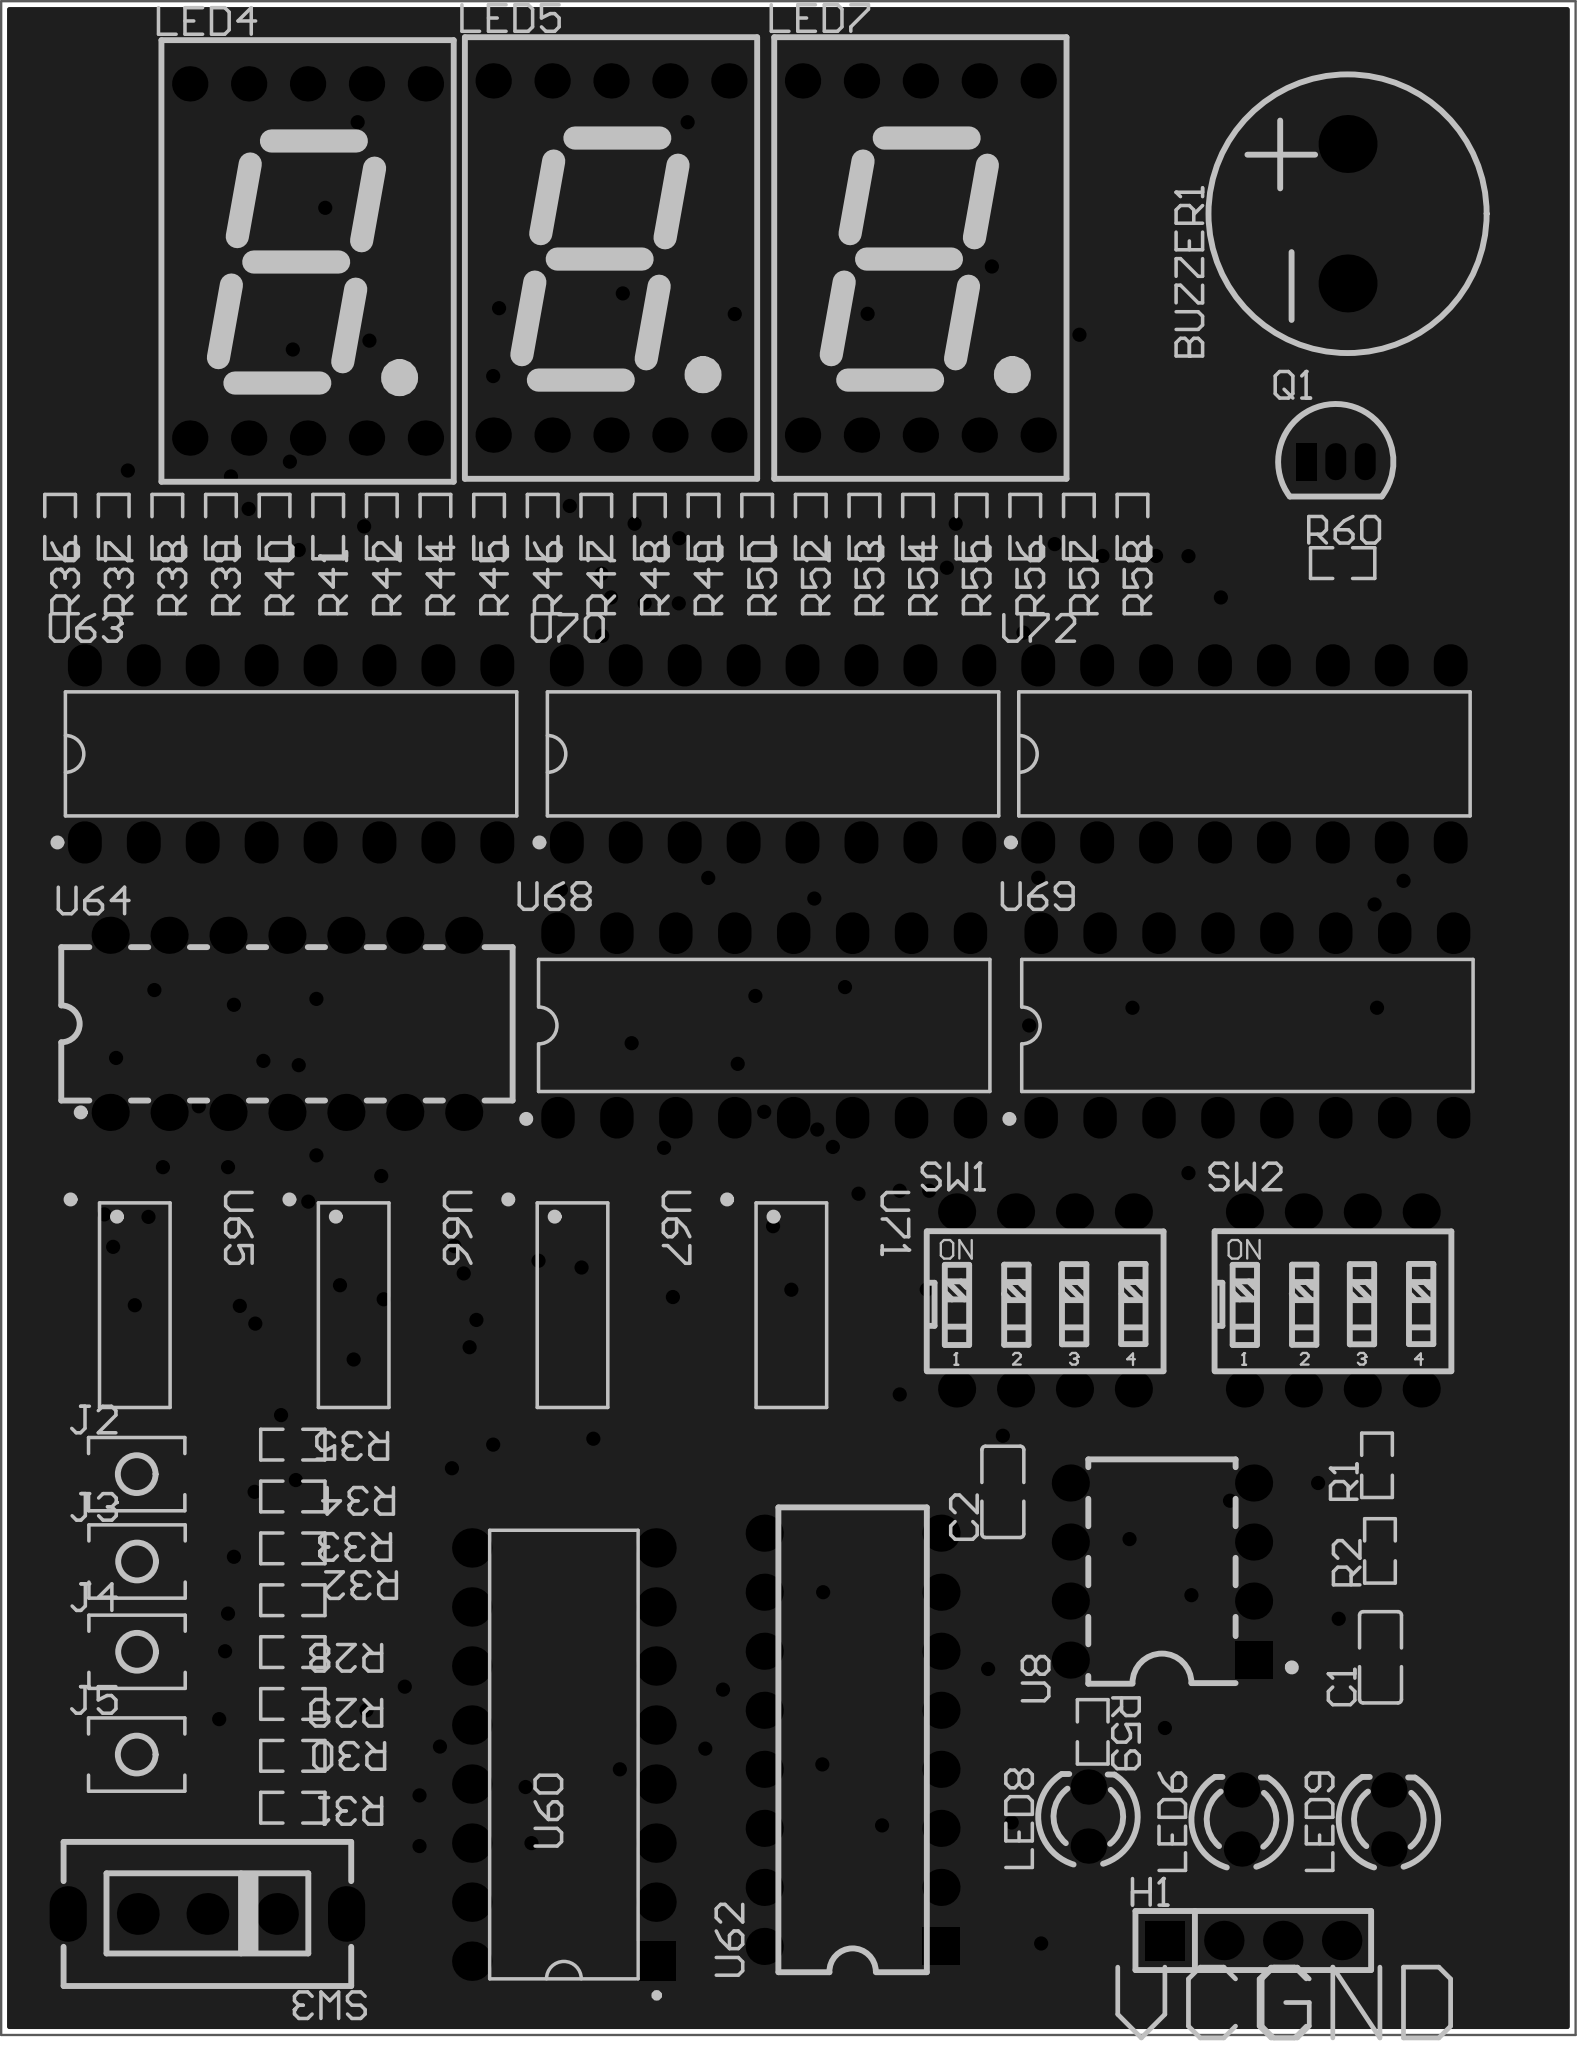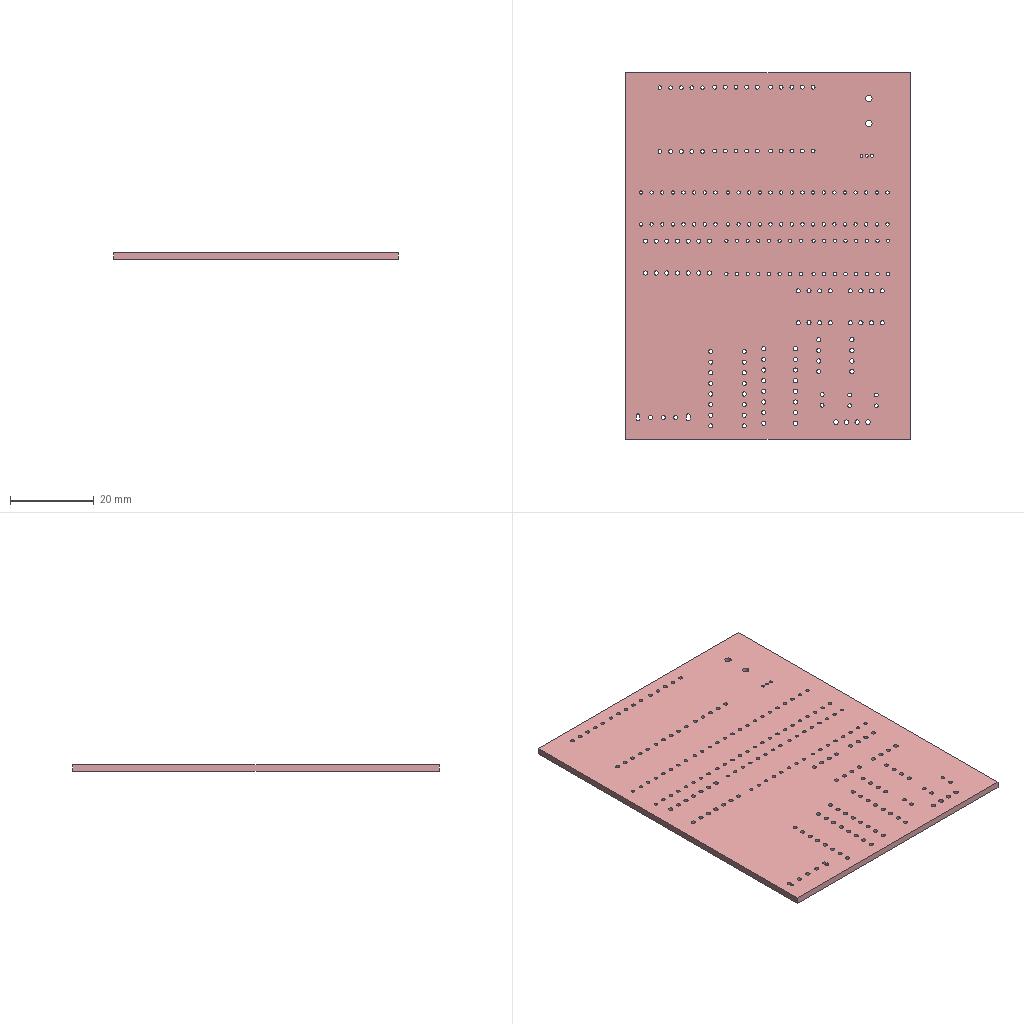Circuit board layout | Altium Designer | box 67.9 x 87.5 x 1.6 mm
Layer stack:
# Altium Designer layer stack of  (unit mm; dielectric type: 0 none, 1 core, 2 prepreg, 3 surface material)
index,name,kind,layer,copper_thickness_mm,dielectric_type,dielectric_thickness_mm,dielectric_material,dielectric_constant
0,Top Paste Mask Layer,other,,,,,,
1,Top Silkscreen Layer,other,,,,,,
2,Top Solder Mask Layer,dielectric,,,3,0.01,,3.3
3,Top Layer,copper,Top Layer,0.035,,,,
4,Dielectric1,dielectric,,,3,1.51,FR4,4.5
5,Bottom Layer,copper,Bottom Layer,0.035,,,,
6,Bottom Solder Mask Layer,dielectric,,,3,0.01,,3.3
7,Bottom Silkscreen Layer,other,,,,,,
8,Bottom Paste Mask Layer,other,,,,,,
# drill layer pairs: low layer,high layer
drill_pair,Top Layer,Bottom Layer
Part placement:
Designator,Comment,Layer,Footprint,Center-X(mm),Center-Y(mm),Rotation
BUZZER1,buzzer,TopLayer,BUZ-TH_BD12.0-P6.00-D0.9-RD,137.668,157.099,90
C1,100uF,TopLayer,C0805,139.089,94.989,90
C2,10nF,TopLayer,C0805,122.809,102.108,90
J2,Tact switch 3*4*H,TopLayer,SW-SMD_L4.0-W2.9-LS5.0,85.471,102.87,0
J3,Tact switch 3*4*H,TopLayer,SW-SMD_L4.0-W2.9-LS5.0,85.486,99.111,0
J4,Tact switch 3*4*H,TopLayer,SW-SMD_L4.0-W2.9-LS5.0,85.486,95.227,0
J5,Tact switch 3*4*H,TopLayer,SW-SMD_L4.0-W2.9-LS5.0,85.471,90.805,0
LED4,,TopLayer,LED-SEG-TH_10P-L12.6-W19.0-P2.54-S15.24-BL,92.837,155.067,0
LED5,,TopLayer,LED-SEG-TH_10P-L12.6-W19.0-P2.54-S15.24-BL,105.918,155.194,0
LED6,,TopLayer,LED_TH-3mm,133.096,88.011,90
LED7,,TopLayer,LED-SEG-TH_10P-L12.6-W19.0-P2.54-S15.24-BL,119.253,155.194,0
LED8,,TopLayer,LED_TH-3mm,126.492,88.138,90
Q1,2N2222A,TopLayer,TO-92-3_L4.9-W3.7-P1.27-L,137.16,146.431,0
R1,10k,TopLayer,R0603,138.938,103.251,90
R2,2.2k,TopLayer,R0603,139.065,99.568,90
R28,10k,TopLayer,R0603,92.202,95.214,180
R29,10k,TopLayer,R0603,92.202,92.982,180
R30,10k,TopLayer,R0603,92.202,90.751,180
R31,10k,TopLayer,R0603,92.202,88.519,180
R32,10k,TopLayer,R0603,92.202,97.445,180
R33,10k,TopLayer,R0603,92.202,99.677,180
R34,10k,TopLayer,R0603,92.202,101.908,180
R35,10k,TopLayer,R0603,92.202,104.14,180
R36,330,TopLayer,R0603,82.169,143.637,90
R37,330,TopLayer,R0603,84.48,143.637,90
R38,330,TopLayer,R0603,86.792,143.637,90
R39,330,TopLayer,R0603,89.103,143.637,90
R40,330,TopLayer,R0603,91.415,143.637,90
R41,330,TopLayer,R0603,93.726,143.637,90
R42,330,TopLayer,R0603,96.037,143.637,90
R44,330,TopLayer,R0603,98.349,143.637,90
R45,330,TopLayer,R0603,100.66,143.637,90
R46,330,TopLayer,R0603,102.972,143.637,90
R47,330,TopLayer,R0603,105.283,143.637,90
R48,330,TopLayer,R0603,107.594,143.637,90
R49,330,TopLayer,R0603,109.906,143.637,90
R50,330,TopLayer,R0603,112.217,143.637,90
R52,330,TopLayer,R0603,114.529,143.637,90
R53,330,TopLayer,R0603,116.84,143.637,90
R54,330,TopLayer,R0603,119.151,143.637,90
R55,330,TopLayer,R0603,121.463,143.637,90
R56,330,TopLayer,R0603,123.774,143.637,90
R57,330,TopLayer,R0603,126.086,143.637,90
R58,330,TopLayer,R0603,128.397,143.637,90
R59,500,TopLayer,R0603,126.681,91.783,270
R60,2k,TopLayer,R0603,137.457,142.066,0
SW1,DIP switch EI-04,TopLayer,SW-TH_DIPSWITCHEI-04,124.625,110.344,0
SW2,DIP switch EI-04,TopLayer,SW-TH_DIPSWITCHEI-04,137.033,110.344,0
U8,NE555PE4,TopLayer,PDIP-8_L9.6-W6.4-P2.54-LS7.9-BL-1,129.667,98.679,90
U60,SN74148N,TopLayer,PDIP-16_L19.3-W6.4-P2.54-LS7.9-BL,103.886,90.805,90
U62,74279N,TopLayer,DIP-16_L19.8-W6.5-P2.54-LS7.6-BL,116.332,91.44,90
U63,SN74LS48N,TopLayer,DIP-16_L19.3-W6.4-P2.54-LS7.6-BL,92.126,133.858,0
U64,SN74LS00N(LX),TopLayer,PDIP-14_L19.3-W6.4-P2.54-LS7.9-BL,91.948,122.244,0
U65,SN74LS04DR,TopLayer,SOIC-14_L8.7-W3.9-P1.27-LS6.0-BL,85.39,110.139,270
U66,SN74LS08DR(LX),TopLayer,SOIC-14_L8.7-W3.9-P1.27-LS6.0-BL,94.824,110.139,270
U67,SN74LS32DR,TopLayer,SOIC-14_L8.7-W3.9-P1.27-LS6.0-BL,104.258,110.139,270
U68,SN74LS192N(LX),TopLayer,PDIP-16_L19.3-W6.4-P2.54-LS7.94-BL,112.522,122.174,0
U69,SN74LS192N(LX),TopLayer,PDIP-16_L19.3-W6.4-P2.54-LS7.94-BL,133.35,122.174,0
U70,SN74LS48N,TopLayer,DIP-16_L19.3-W6.4-P2.54-LS7.6-BL,112.903,133.858,0
U71,SN74LS04DR,TopLayer,SOIC-14_L8.7-W3.9-P1.27-LS6.0-BL,113.692,110.139,270
U72,SN74LS48N,TopLayer,DIP-16_L19.3-W6.4-P2.54-LS7.6-BL,133.223,133.858,0
LED9,,TopLayer,LED_TH-3mm,139.446,88.011,90
SW3,SWITCH-slide three-pin two-position,TopLayer,SW-TH_C9900003112,88.519,83.947,180
H1,,TopLayer,HDR-TH_4P-P2.54-V-M,133.604,82.804,0
Pad and via stacks:
# Altium Designer via and pad stacks of  (unit mm). Each distinct definition once, with the count of objects using it.
# via: kind,start_layer,end_layer,hole_mm,diameter_mm,mode(0 simple;1 top-mid-bottom;2 full stack),diameter_per_layer,count,example_net
# pad: kind,layer,hole_mm,hole_type(0 round;1 square;2 slot),plating,top_size,top_shape(1 round;2 rect;3 octagon;9 rounded rect),mid_size,bottom_size,mode,footprint,size_per_layer,count,example
pad,Multi-Layer,1.5,0,plated,2.5x2.5,1,2.5x2.5,2.5x2.5,0,BUZ-TH_BD12.0-P6.00-D0.9-RD,,2,BUZZER1.1
pad,Multi-Layer,0.9144,0,plated,1.524x1.524,1,1.524x1.524,1.524x1.524,0,LED-SEG-TH_10P-L12.6-W19.0-P2.54-S15.24-BL,,30,LED4.1
pad,Multi-Layer,0.9144,0,plated,1.524x1.524,1,1.524x1.524,1.524x1.524,0,LED_TH-3mm,,6,LED6.1
pad,Multi-Layer,0.7,0,plated,0.9x1.6,1,0.9x1.6,0.9x1.6,0,TO-92-3_L4.9-W3.7-P1.27-L,,2,Q1.3
pad,Multi-Layer,0.7,0,plated,0.9x1.6,2,0.9x1.6,0.9x1.6,0,TO-92-3_L4.9-W3.7-P1.27-L,,1,Q1.1
pad,Multi-Layer,1,0,plated,1.6x1.6,1,1.6x1.6,1.6x1.6,0,SW-TH_DIPSWITCHEI-04,,16,SW1.1
pad,Multi-Layer,1,0,plated,1.6x1.6,1,1.6x1.6,1.6x1.6,0,PDIP-8_L9.6-W6.4-P2.54-LS7.9-BL-1,,7,U8.8
pad,Multi-Layer,1,0,plated,1.6x1.6,2,1.6x1.6,1.6x1.6,0,PDIP-8_L9.6-W6.4-P2.54-LS7.9-BL-1,,1,U8.1
pad,Multi-Layer,1,0,plated,1.7x1.7,2,1.7x1.7,1.7x1.7,0,PDIP-16_L19.3-W6.4-P2.54-LS7.9-BL,,1,U60.1
pad,Multi-Layer,1,0,plated,1.7x1.7,1,1.7x1.7,1.7x1.7,0,PDIP-16_L19.3-W6.4-P2.54-LS7.9-BL,,15,U60.2
pad,Multi-Layer,1,0,plated,1.6x1.6,1,1.6x1.6,1.6x1.6,0,DIP-16_L19.8-W6.5-P2.54-LS7.6-BL,,15,U62.16
pad,Multi-Layer,1,0,plated,1.6x1.6,2,1.6x1.6,1.6x1.6,0,DIP-16_L19.8-W6.5-P2.54-LS7.6-BL,,1,U62.1
pad,Multi-Layer,0.8,0,plated,1.46x1.825,1,1.46x1.825,1.46x1.825,0,DIP-16_L19.3-W6.4-P2.54-LS7.6-BL,,48,U63.9
pad,Multi-Layer,1,0,plated,1.6x1.6,1,1.6x1.6,1.6x1.6,0,PDIP-14_L19.3-W6.4-P2.54-LS7.9-BL,,14,U64.9
pad,Multi-Layer,0.8,0,plated,1.44x1.8,1,1.44x1.8,1.44x1.8,0,PDIP-16_L19.3-W6.4-P2.54-LS7.94-BL,,32,U68.1
pad,Multi-Layer,0.9,2,plated,1.6x2.4,1,1.6x2.4,1.6x2.4,0,SW-TH_C9900003112,,2,SW3.EH
pad,Multi-Layer,1,0,plated,1.8x1.8,1,1.8x1.8,1.8x1.8,0,SW-TH_C9900003112,,3,SW3.3
pad,Multi-Layer,1.1,0,plated,1.7x1.7,2,1.7x1.7,1.7x1.7,0,HDR-TH_4P-P2.54-V-M,,1,H1.1
pad,Multi-Layer,1.1,0,plated,1.7x1.7,1,1.7x1.7,1.7x1.7,0,HDR-TH_4P-P2.54-V-M,,3,H1.2
pad,Top Layer,0,0,plated,1.41x1.35,2,1.41x1.35,1.41x1.35,0,C0805,,4,C1.2
pad,Top Layer,0,0,plated,1.53x1.36,2,1.53x1.36,1.53x1.36,0,SW-SMD_L4.0-W2.9-LS5.0,,8,J2.1
pad,Top Layer,0,0,plated,0.8065x0.864,2,0.8065x0.864,0.8065x0.864,0,R0603,,66,R1.2
pad,Top Layer,0,0,plated,0.574x2.038,1,0.574x2.038,0.574x2.038,0,SOIC-14_L8.7-W3.9-P1.27-LS6.0-BL,,56,U65.1
via,Top Layer,Bottom Layer,0.3048,0.61,0,,119,$1N11481
via,Top Layer,Bottom Layer,0.3048,0.6096,0,,1,VCC
Copper pours:
name,layer,net,type(0 solid;1 hatched;2 none)
Bottom Layer-GND,Bottom Layer,GND,0
Top Layer-GND,Top Layer,GND,0